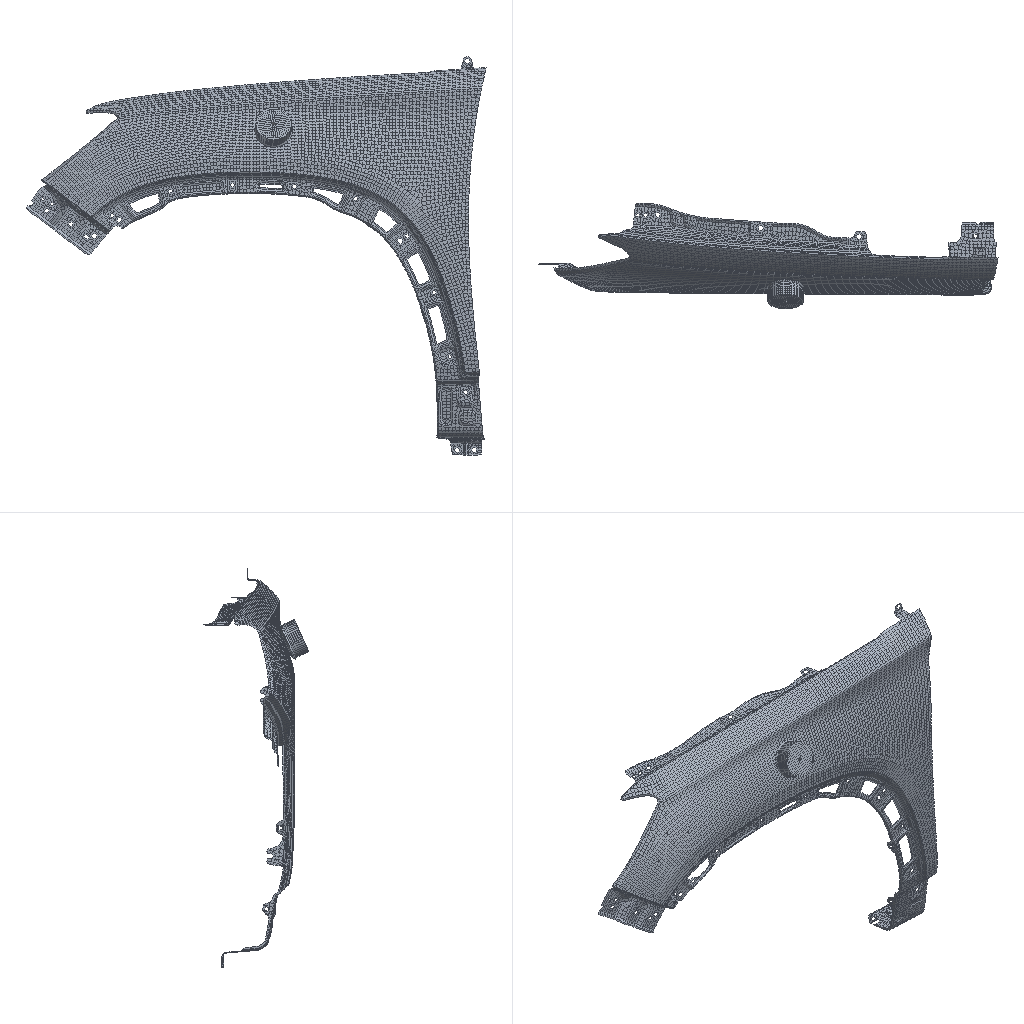Simulation study | abaqus
Set-up summary:
category,name,step,type,value,unit,region
solver,abaqus
solver,version,,,Abaqus/Standard 3DEXPERIENCE R2017x
units,not stated in the deck,,not stated
analysis,deck,,static,static
load_step,load,load,static,nlgeom=True
load_step,unload,unload,static,nlgeom=True
contact,interactions,,,general=0 pairs=1 ties=0
load_step,requested,,,2
mesh,nodes,,,12240
mesh,elements,,,11562
element_type,S3,,shell,568
element_type,S4,,shell,9090
element_type,C3D8,,solid,1664
element_type,C3D8H,,solid,240
load,load commands in deck,,count,1
bc,support commands in deck,,count,14
material,HC180Y,,in results
material,MAT-STEEL,,in results
material,RUBBER,,in results
check,setup vs results,,match,"per instance, exact: element labels, types and connectivity; labels of the nodes the elements use; coordinates not compared"
Abaqus input file, long lists of numbers shortened:
**
** ABAQUS Input Deck Generated by HyperMesh Version  : 14.0.0.88
** Generated using HyperMesh-Abaqus Template Version : 14.0
**
**   Template:  ABAQUS/STANDARD 3D
**
*NODE
         1,  -435.848       ,  -889.15        ,  300.419
         2,  -437.816       ,  -889.15        ,  297.793
** (12237 more lines like these left out)
**HMNAME SYSTEMCOL auto1,         1,    4
*SYSTEM
55.106, -950.955, 541.11, 54.119, -951.017, 540.965
54.948, -950.55, 542.011
*NODE, SYSTEM=R
   2133045,  0.0            ,  0.0            ,  0.0
**HWCOLOR COMP        371    21
*ELEMENT,TYPE=S3,ELSET=KX63_F08-8403101_HC180Y_T070
        13,        27,      3741,      2715
        37,      7291,      7290,       590
** (566 more lines like these left out)
**HWCOLOR COMP        371    21
*ELEMENT,TYPE=S4,ELSET=KX63_F08-8403101_HC180Y_T070
         1,         4,         5,         6,         3
         2,       581,       611,        31,       588
** (9088 more lines like these left out)
**HWCOLOR COMP          1    21
*ELEMENT,TYPE=C3D8,ELSET=impactor
   2127998,    839956,    839918,    839973,    839922,    839778,    839312,    839786,
    839315
** (3326 more lines like these left out)
**HWCOLOR COMP          2    55
*ELEMENT,TYPE=C3D8H,ELSET=rubber
     14376,    838547,    838651,    838694,    838463,    838914,    838951,    839220,
    838890
** (478 more lines like these left out)
**HWNAME COMP    2000070 FRONT_RH_REB2
**HWCOLOR COMP    2000070    29
*KINEMATIC COUPLING,REF NODE=2133045
    838213,1,6
    838215,1,6
    838216,1,6
    838220,1,6
    838224,1,6
    838230,1,6
    838236,1,6
    838237,1,6
    838238,1,6
    838239,1,6
    838242,1,6
    838244,1,6
    838247,1,6
    838248,1,6
    838250,1,6
    838251,1,6
    838252,1,6
    838253,1,6
    838256,1,6
    838257,1,6
    838259,1,6
    838260,1,6
    838272,1,6
    838275,1,6
    838278,1,6
    838282,1,6
    838284,1,6
    838299,1,6
    838301,1,6
    838302,1,6
    838305,1,6
    838307,1,6
    838308,1,6
    838313,1,6
    838315,1,6
    838319,1,6
    838320,1,6
    838321,1,6
    838324,1,6
    838325,1,6
** (224 more lines like these left out)
**HWNAME COMP        370 RB2
**HWCOLOR COMP        370    18
*COUPLING, REF NODE=839102, CONSTRAINT NAME="HM_coupkin_20971", SURFACE="HM_coupkin_surface_20971"
*KINEMATIC
1,6
*SURFACE, NAME ="HM_coupkin_surface_20971", TYPE = NODE
       349, 1
       350, 1
      6702, 1
      6704, 1
      6707, 1
      6709, 1
      6712, 1
      6714, 1
     11735, 1
     11737, 1
     11738, 1
     11741, 1
     11743, 1
     11744, 1
     11754, 1
     11837, 1
     11869, 1
     11870, 1
     11879, 1
     12733, 1
**HWNAME COMP        370 RB2
**HWCOLOR COMP        370    18
*COUPLING, REF NODE=839103, CONSTRAINT NAME="HM_coupkin_20972", SURFACE="HM_coupkin_surface_20972"
*KINEMATIC
1,6
*SURFACE, NAME ="HM_coupkin_surface_20972", TYPE = NODE
       321, 1
       322, 1
      6671, 1
      6678, 1
     12483, 1
     12560, 1
     12561, 1
     12562, 1
     12563, 1
     12568, 1
     12569, 1
     12573, 1
     12574, 1
     12575, 1
     12584, 1
     12585, 1
     12591, 1
     12593, 1
     12600, 1
     12611, 1
**HWNAME COMP        370 RB2
**HWCOLOR COMP        370    18
*COUPLING, REF NODE=839104, CONSTRAINT NAME="HM_coupkin_20973", SURFACE="HM_coupkin_surface_20973"
*KINEMATIC
1,6
*SURFACE, NAME ="HM_coupkin_surface_20973", TYPE = NODE
      7110, 1
      7113, 1
      7118, 1
      7119, 1
      7129, 1
**HWNAME COMP        370 RB2
**HWCOLOR COMP        370    18
*COUPLING, REF NODE=839105, CONSTRAINT NAME="HM_coupkin_20974", SURFACE="HM_coupkin_surface_20974"
*KINEMATIC
1,6
*SURFACE, NAME ="HM_coupkin_surface_20974", TYPE = NODE
     11441, 1
     11445, 1
     11446, 1
     11448, 1
     11451, 1
**HWNAME COMP        370 RB2
**HWCOLOR COMP        370    18
*COUPLING, REF NODE=839106, CONSTRAINT NAME="HM_coupkin_20976", SURFACE="HM_coupkin_surface_20976"
*KINEMATIC
1,6
*SURFACE, NAME ="HM_coupkin_surface_20976", TYPE = NODE
      7300, 1
      7326, 1
      7330, 1
      7331, 1
      7333, 1
      7334, 1
      7335, 1
      7337, 1
     11729, 1
     11749, 1
     11751, 1
     11755, 1
     11756, 1
     11757, 1
     11771, 1
     12043, 1
     12068, 1
     12111, 1
     12116, 1
     12220, 1
**HWNAME COMP        370 RB2
**HWCOLOR COMP        370    18
*COUPLING, REF NODE=839108, CONSTRAINT NAME="HM_coupkin_20983", SURFACE="HM_coupkin_surface_20983"
*KINEMATIC
1,6
*SURFACE, NAME ="HM_coupkin_surface_20983", TYPE = NODE
        36, 1
        49, 1
        78, 1
        80, 1
        81, 1
        82, 1
        85, 1
        91, 1
       105, 1
       107, 1
      7750, 1
      7761, 1
     11457, 1
     11458, 1
     11460, 1
     11461, 1
     11462, 1
     11463, 1
     11464, 1
     11588, 1
    839107, 1
**HWNAME COMP        370 RB2
**HWCOLOR COMP        370    18
*COUPLING, REF NODE=839109, CONSTRAINT NAME="HM_coupkin_20984", SURFACE="HM_coupkin_surface_20984"
*KINEMATIC
1,6
*SURFACE, NAME ="HM_coupkin_surface_20984", TYPE = NODE
      7612, 1
      7613, 1
      7630, 1
     12349, 1
     12580, 1
     12581, 1
     12587, 1
     12588, 1
     12596, 1
     12598, 1
     12601, 1
     12602, 1
     12603, 1
     12604, 1
     12605, 1
     12606, 1
     12607, 1
     12608, 1
     12609, 1
     12610, 1
**HWNAME COMP        370 RB2
**HWCOLOR COMP        370    18
*COUPLING, REF NODE=839110, CONSTRAINT NAME="HM_coupkin_20985", SURFACE="HM_coupkin_surface_20985"
*KINEMATIC
1,6
*SURFACE, NAME ="HM_coupkin_surface_20985", TYPE = NODE
      7451, 1
      7458, 1
     12511, 1
     12514, 1
     12519, 1
     12524, 1
     12525, 1
     12530, 1
     12531, 1
     12536, 1
     12541, 1
     12543, 1
     12546, 1
     12548, 1
     12552, 1
     12553, 1
     12557, 1
     12558, 1
     12576, 1
     12577, 1
**HWNAME COMP        370 RB2
**HWCOLOR COMP        370    18
*COUPLING, REF NODE=839111, CONSTRAINT NAME="HM_coupkin_20986", SURFACE="HM_coupkin_surface_20986"
*KINEMATIC
1,6
*SURFACE, NAME ="HM_coupkin_surface_20986", TYPE = NODE
       675, 1
       677, 1
       678, 1
       682, 1
     12430, 1
     12431, 1
     12435, 1
     12436, 1
     12441, 1
     12442, 1
     12444, 1
     12445, 1
     12446, 1
     12447, 1
     12448, 1
     12449, 1
**HWNAME COMP        370 RB2
**HWCOLOR COMP        370    18
*COUPLING, REF NODE=839144, CONSTRAINT NAME="HM_coupkin_21050", SURFACE="HM_coupkin_surface_21050"
*KINEMATIC
1,6
*SURFACE, NAME ="HM_coupkin_surface_21050", TYPE = NODE
       977, 1
       978, 1
       979, 1
       984, 1
       995, 1
       996, 1
       998, 1
      1018, 1
     12451, 1
     12452, 1
     12453, 1
     12454, 1
     12455, 1
     12456, 1
     12457, 1
     12458, 1
**HWNAME COMP        370 RB2
**HWCOLOR COMP        370    18
*COUPLING, REF NODE=839145, CONSTRAINT NAME="HM_coupkin_21051", SURFACE="HM_coupkin_surface_21051"
*KINEMATIC
1,6
*SURFACE, NAME ="HM_coupkin_surface_21051", TYPE = NODE
       883, 1
       888, 1
       889, 1
       893, 1
       895, 1
       896, 1
       898, 1
       900, 1
       902, 1
       903, 1
       906, 1
       907, 1
       909, 1
       910, 1
       914, 1
     11727, 1
     11775, 1
     11781, 1
     12460, 1
     12463, 1
**HWNAME COMP        370 RB2
**HWCOLOR COMP        370    18
*COUPLING, REF NODE=839146, CONSTRAINT NAME="HM_coupkin_21052", SURFACE="HM_coupkin_surface_21052"
*KINEMATIC
1,6
*SURFACE, NAME ="HM_coupkin_surface_21052", TYPE = NODE
       997, 1
      1008, 1
      1016, 1
      1021, 1
     12078, 1
     12079, 1
     12459, 1
     12461, 1
     12462, 1
     12467, 1
     12468, 1
     12469, 1
**HMNAME SYSTEMCOL auto1,         1,    4
*TRANSFORM, TYPE=R, NSET=HM_auto_transform_208C35
-0.9875, -0.06149, -0.1453,  -0.1577,  0.4052 ,  0.9005
**HMORIENT ORIGIN  55.106,-950.955,541.11
**HM_PROP_ID         38
**HM_comp_by_property "impactor"    56
*SOLID SECTION, ELSET=impactor, MATERIAL=mat-steel
**HM_PROP_ID         39
**HM_comp_by_property "rubber"    56
*SOLID SECTION, ELSET=rubber, MATERIAL=rubber
**HM_PROP_ID         25
**HM_comp_by_property "KX63_F08-8403101_HC180Y_T070"     4
*SHELL SECTION, ELSET=KX63_F08-8403101_HC180Y_T070, MATERIAL=HC180Y
0.7       ,
*NSET, NSET=node
   2133045,
*ELSET, ELSET=master
      3167,      3172,      3175,      3177,      3180,      3182,      3185,      3187,
      3190,      3192,      3195,      3197,      3200,      3202,      3205,      3207,
** (16 more lines like these left out)
*NSET, NSET=HM_auto_transform_208C35
   2133045,
**HMNAME MATS          2 HC180Y     3
*MATERIAL, NAME=HC180Y
*DENSITY
7.8500E-09,0.0
*ELASTIC, TYPE = ISOTROPIC
210000.0  ,0.3       ,0.0
*PLASTIC
239.2     ,0.0       ,0.0
260.6     ,0.0092    ,0.0
281.1     ,0.0149    ,0.0
310.0     ,0.03      ,0.0
329.1     ,0.0431    ,0.0
346.0     ,0.0575    ,0.0
361.8     ,0.074     ,0.0
374.9     ,0.0907    ,0.0
390.9     ,0.115     ,0.0
405.6     ,0.1426    ,0.0
416.3     ,0.1661    ,0.0
423.2     ,0.183     ,0.0
432.6     ,0.2086    ,0.0
439.3     ,0.2298    ,0.0
442.9     ,0.2487    ,0.0
**HMNAME MATS          3 mat-steel     4
*MATERIAL, NAME=mat-steel
*DENSITY
7.8500E-09,0.0
*ELASTIC, TYPE = ISOTROPIC
210000.0  ,0.3       ,0.0
**HMNAME MATS        115 rubber     5
*MATERIAL, NAME=rubber
*DENSITY
1.0000E-09,0.0
*HYPERELASTIC, N = 2,POLYNOMIAL
0.3559   ,-0.2859  ,1.354    ,0.   ,0.   ,0.   ,0.   ,
**HMNAME PROPERTY         40 FRIC
*SURFACE INTERACTION, NAME = FRIC
*FRICTION
0.2       ,0.0       ,0.0       ,0.0
**HMNAME GROUPS          3 cp
*CONTACT PAIR, INTERACTION=FRIC, ADJUST=0.05, TYPE=SURFACE TO SURFACE
slave, master
*SURFACE, NAME = slave, TYPE = ELEMENT
     14376, S2
     14377, S2
    810251, S2
     14378, S2
     14379, S2
     14380, S2
     14385, S2
    810296, S2
     14381, S2
    810252, S2
     14417, S2
     14382, S2
     14387, S2
    810253, S2
     14383, S2
     14384, S2
     14391, S2
     14386, S2
     14388, S2
     14422, S2
     14389, S2
     14390, S2
    810287, S2
     14392, S2
     14496, S2
     14393, S2
     14394, S2
    810267, S2
     14395, S2
     14396, S2
     14397, S2
     14398, S2
     14399, S2
    810254, S2
     14400, S2
     14401, S2
    810255, S2
     14476, S2
     21055, S2
     14402, S2
** (200 more lines like these left out)
*SURFACE, NAME = master, TYPE = ELEMENT
master,SNEG
**HWNAME LOADCOL          1 spc
**HWCOLOR LOADCOL          1    18
*BOUNDARY
    839111,1,6,
    839110,1,6,
    839102,1,6,
    839103,1,6,
    839106,1,6,
    839108,1,6,
    839146,1,6,
    839144,1,6,
    839109,1,6,
    839145,1,6,
    839105,1,6,
    839104,1,6,
   2133045,1,2,
   2133045,4,6,
**HMNAME LOADSTEP          1 load
*STEP, NAME = load, NLGEOM = YES
*STATIC
0.1       ,1.0       ,1.0000E-06,0.2
*MONITOR, DOF =     3, NODE = node
**HWNAME LOADCOL          2 load
**HWCOLOR LOADCOL          2     6
*CLOAD
   2133045,3,400.0
*OUTPUT, FIELD
*NODE OUTPUT
U,
CF,
*ELEMENT OUTPUT
S,
E,
PEEQ,
*END STEP
**HMNAME LOADSTEP          2 unload
*STEP, NAME = unload, NLGEOM = YES
*STATIC
0.1       ,1.0       ,1.0000E-06,0.2
*MONITOR, DOF =     3, NODE = node
**HWNAME LOADCOL          3 unload
**HWCOLOR LOADCOL          3    33
*CLOAD, OP=NEW
*OUTPUT, FIELD
*NODE OUTPUT
U,
CF,
*ELEMENT OUTPUT
S,
E,
PEEQ,
*END STEP
*****
Results summary:
result,step,,completed,increments=16 time=1.0/1.0
result,step,,completed,increments=16 time=1.0/1.0
result,analysis,,,static
result,last_loadstep,,,2
result,analysis steps,,count,2
result,primary field,,,"U, UR"